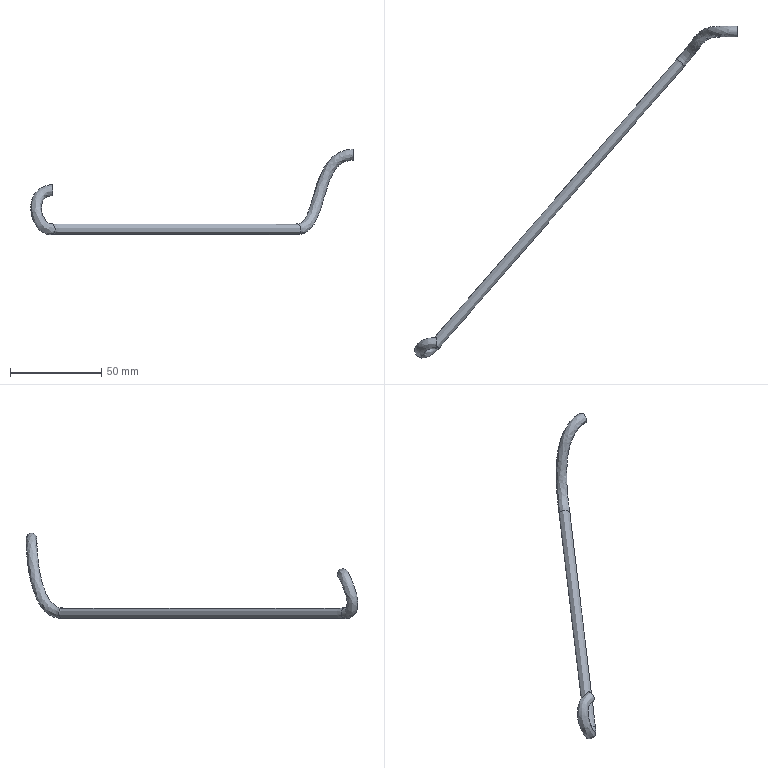Part | NX | features solid 2 | 1 solid | 8 faces | box 177.179 x 182.356 x 47.005 mm | volume 4713 mm3 | spline 6 | plane 2